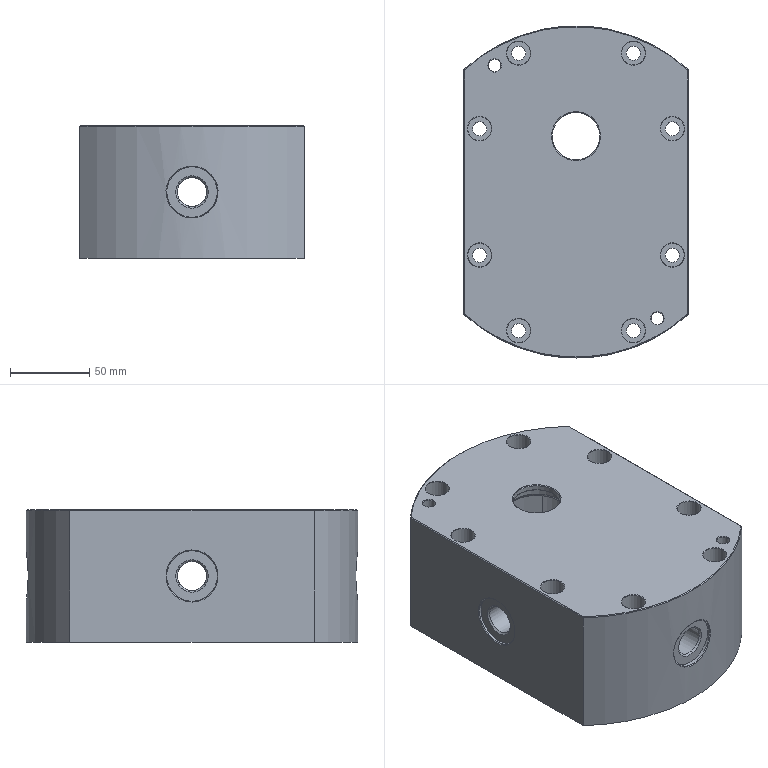NC program | NX | posted with a generic post | part box 142 x 210 x 84 mm
Lines 1 to 961 of 7150:
N10 G17 G21 G94 G90
(FLOOR_WALL_COPY_1 , TOOL : D50)
N12 T02 M6
N14 G54
N16 G17 G0 G90 X-143. Y80.997 B0. C0. S1200 M3
N18 G43 Z30. H2
N20 Z12.658
N22 G94 G1 Z9.658 F1000.
N24 X-140.
N26 X140. F2000.
N28 Y45.498
N30 X-140.
N32 Y9.999
N34 X140.
N36 Y-25.501
N38 X-140.
N40 Y-61.
N42 X140.
N44 X143.
N46 Z12.658
N48 G0 Z30.
N50 X-143. Y80.997
N52 Z12.317
N54 G1 Z9.317 F1000.
N56 X-140.
N58 X140. F2000.
N60 Y45.498
N62 X-140.
N64 Y9.999
N66 X140.
N68 Y-25.501
N70 X-140.
N72 Y-61.
N74 X140.
N76 X143.
N78 Z12.317
N80 G0 Z30.
N82 X-143. Y80.997
N84 Z11.976
N86 G1 Z8.976 F1000.
N88 X-140.
N90 X140. F2000.
N92 Y45.498
N94 X-140.
N96 Y9.999
N98 X140.
N100 Y-25.501
N102 X-140.
N104 Y-61.
N106 X140.
N108 X143.
N110 Z11.976
N112 G0 Z30.
N114 X-143. Y80.997
N116 Z11.634
N118 G1 Z8.634 F1000.
N120 X-140.
N122 X140. F2000.
N124 Y45.498
N126 X-140.
N128 Y9.999
N130 X140.
N132 Y-25.501
N134 X-140.
N136 Y-61.
N138 X140.
N140 X143.
N142 Z11.634
N144 G0 Z30.
N146 X-143. Y80.997
N148 Z11.293
N150 G1 Z8.293 F1000.
N152 X-140.
N154 X140. F2000.
N156 Y45.498
N158 X-140.
N160 Y9.999
N162 X140.
N164 Y-25.501
N166 X-140.
N168 Y-61.
N170 X140.
N172 X143.
N174 Z11.293
N176 G0 Z30.
N178 X-143. Y80.997
N180 Z10.951
N182 G1 Z7.951 F1000.
N184 X-140.
N186 X140. F2000.
N188 Y45.498
N190 X-140.
N192 Y9.999
N194 X140.
N196 Y-25.501
N198 X-140.
N200 Y-61.
N202 X140.
N204 X143.
N206 Z10.951
N208 G0 Z30.
N210 X-143. Y80.997
N212 Z10.61
N214 G1 Z7.61 F1000.
N216 X-140.
N218 X140. F2000.
N220 Y45.498
N222 X-140.
N224 Y9.999
N226 X140.
N228 Y-25.501
N230 X-140.
N232 Y-61.
N234 X140.
N236 X143.
N238 Z10.61
N240 G0 Z30.
N242 X-143. Y80.997
N244 Z10.269
N246 G1 Z7.269 F1000.
N248 X-140.
N250 X140. F2000.
N252 Y45.498
N254 X-140.
N256 Y9.999
N258 X140.
N260 Y-25.501
N262 X-140.
N264 Y-61.
N266 X140.
N268 X143.
N270 Z10.269
N272 G0 Z30.
N274 X-143. Y80.997
N276 Z9.927
N278 G1 Z6.927 F1000.
N280 X-140.
N282 X140. F2000.
N284 Y45.498
N286 X-140.
N288 Y9.999
N290 X140.
N292 Y-25.501
N294 X-140.
N296 Y-61.
N298 X140.
N300 X143.
N302 Z9.927
N304 G0 Z30.
N306 X-143. Y80.997
N308 Z9.586
N310 G1 Z6.586 F1000.
N312 X-140.
N314 X140. F2000.
N316 Y45.498
N318 X-140.
N320 Y9.999
N322 X140.
N324 Y-25.501
N326 X-140.
N328 Y-61.
N330 X140.
N332 X143.
N334 Z9.586
N336 G0 Z30.
N338 X-143. Y80.997
N340 Z9.245
N342 G1 Z6.245 F1000.
N344 X-140.
N346 X140. F2000.
N348 Y45.498
N350 X-140.
N352 Y9.999
N354 X140.
N356 Y-25.501
N358 X-140.
N360 Y-61.
N362 X140.
N364 X143.
N366 Z9.245
N368 G0 Z30.
N370 X-143. Y80.997
N372 Z8.903
N374 G1 Z5.903 F1000.
N376 X-140.
N378 X140. F2000.
N380 Y45.498
N382 X-140.
N384 Y9.999
N386 X140.
N388 Y-25.501
N390 X-140.
N392 Y-61.
N394 X140.
N396 X143.
N398 Z8.903
N400 G0 Z30.
N402 X-143. Y80.997
N404 Z8.562
N406 G1 Z5.562 F1000.
N408 X-140.
N410 X140. F2000.
N412 Y45.498
N414 X-140.
N416 Y9.999
N418 X140.
N420 Y-25.501
N422 X-140.
N424 Y-61.
N426 X140.
N428 X143.
N430 Z8.562
N432 G0 Z30.
N434 X-143. Y80.997
N436 Z8.221
N438 G1 Z5.221 F1000.
N440 X-140.
N442 X140. F2000.
N444 Y45.498
N446 X-140.
N448 Y9.999
N450 X140.
N452 Y-25.501
N454 X-140.
N456 Y-61.
N458 X140.
N460 X143.
N462 Z8.221
N464 G0 Z30.
N466 X-143. Y80.997
N468 Z7.879
N470 G1 Z4.879 F1000.
N472 X-140.
N474 X140. F2000.
N476 Y45.498
N478 X-140.
N480 Y9.999
N482 X140.
N484 Y-25.501
N486 X-140.
N488 Y-61.
N490 X140.
N492 X143.
N494 Z7.879
N496 G0 Z30.
N498 X-143. Y80.997
N500 Z7.538
N502 G1 Z4.538 F1000.
N504 X-140.
N506 X140. F2000.
N508 Y45.498
N510 X-140.
N512 Y9.999
N514 X140.
N516 Y-25.501
N518 X-140.
N520 Y-61.
N522 X140.
N524 X143.
N526 Z7.538
N528 G0 Z30.
N530 X-143. Y80.997
N532 Z7.196
N534 G1 Z4.196 F1000.
N536 X-140.
N538 X140. F2000.
N540 Y45.498
N542 X-140.
N544 Y9.999
N546 X140.
N548 Y-25.501
N550 X-140.
N552 Y-61.
N554 X140.
N556 X143.
N558 Z7.196
N560 G0 Z30.
N562 X-143. Y80.997
N564 Z6.855
N566 G1 Z3.855 F1000.
N568 X-140.
N570 X140. F2000.
N572 Y45.498
N574 X-140.
N576 Y9.999
N578 X140.
N580 Y-25.501
N582 X-140.
N584 Y-61.
N586 X140.
N588 X143.
N590 Z6.855
N592 G0 Z30.
N594 X-143. Y80.997
N596 Z6.514
N598 G1 Z3.514 F1000.
N600 X-140.
N602 X140. F2000.
N604 Y45.498
N606 X-140.
N608 Y9.999
N610 X140.
N612 Y-25.501
N614 X-140.
N616 Y-61.
N618 X140.
N620 X143.
N622 Z6.514
N624 G0 Z30.
N626 X-143. Y80.997
N628 Z6.172
N630 G1 Z3.172 F1000.
N632 X-140.
N634 X140. F2000.
N636 Y45.498
N638 X-140.
N640 Y9.999
N642 X140.
N644 Y-25.501
N646 X-140.
N648 Y-61.
N650 X140.
N652 X143.
N654 Z6.172
N656 G0 Z30.
N658 X-143. Y80.997
N660 Z5.831
N662 G1 Z2.831 F1000.
N664 X-140.
N666 X140. F2000.
N668 Y45.498
N670 X-140.
N672 Y9.999
N674 X140.
N676 Y-25.501
N678 X-140.
N680 Y-61.
N682 X140.
N684 X143.
N686 Z5.831
N688 G0 Z30.
N690 X-143. Y80.997
N692 Z5.49
N694 G1 Z2.49 F1000.
N696 X-140.
N698 X140. F2000.
N700 Y45.498
N702 X-140.
N704 Y9.999
N706 X140.
N708 Y-25.501
N710 X-140.
N712 Y-61.
N714 X140.
N716 X143.
N718 Z5.49
N720 G0 Z30.
N722 X-143. Y80.997
N724 Z5.148
N726 G1 Z2.148 F1000.
N728 X-140.
N730 X140. F2000.
N732 Y45.498
N734 X-140.
N736 Y9.999
N738 X140.
N740 Y-25.501
N742 X-140.
N744 Y-61.
N746 X140.
N748 X143.
N750 Z5.148
N752 G0 Z30.
N754 X-143. Y80.997
N756 Z4.807
N758 G1 Z1.807 F1000.
N760 X-140.
N762 X140. F2000.
N764 Y45.498
N766 X-140.
N768 Y9.999
N770 X140.
N772 Y-25.501
N774 X-140.
N776 Y-61.
N778 X140.
N780 X143.
N782 Z4.807
N784 G0 Z30.
N786 X-143. Y80.997
N788 Z4.465
N790 G1 Z1.465 F1000.
N792 X-140.
N794 X140. F2000.
N796 Y45.498
N798 X-140.
N800 Y9.999
N802 X140.
N804 Y-25.501
N806 X-140.
N808 Y-61.
N810 X140.
N812 X143.
N814 Z4.465
N816 G0 Z30.
N818 X-143. Y80.997
N820 Z4.124
N822 G1 Z1.124 F1000.
N824 X-140.
N826 X140. F2000.
N828 Y45.498
N830 X-140.
N832 Y9.999
N834 X140.
N836 Y-25.501
N838 X-140.
N840 Y-61.
N842 X140.
N844 X143.
N846 Z4.124
N848 G0 Z30.
N850 X-143. Y80.997
N852 Z3.783
N854 G1 Z0.783 F1000.
N856 X-140.
N858 X140. F2000.
N860 Y45.498
N862 X-140.
N864 Y9.999
N866 X140.
N868 Y-25.501
N870 X-140.
N872 Y-61.
N874 X140.
N876 X143.
N878 Z3.783
N880 G0 Z30.
N882 X-143. Y80.997
N884 Z3.441
N886 G1 Z0.441 F1000.
N888 X-140.
N890 X140. F2000.
N892 Y45.498
N894 X-140.
N896 Y9.999
N898 X140.
N900 Y-25.501
N902 X-140.
N904 Y-61.
N906 X140.
N908 X143.
N910 Z3.441
N912 G0 Z30.
N914 X-143. Y80.997
N916 Z3.1
N918 G1 Z0.1 F1000.
N920 X-140.
N922 X140. F2000.
N924 Y45.498
N926 X-140.
N928 Y9.999
N930 X140.
N932 Y-25.501
N934 X-140.
N936 Y-61.
N938 X140.
N940 X143.
N942 Z3.1
N944 G0 Z30.
(FLOOR_WALL_COPY_COPY , TOOL : D50)
N946 X-143. Y80.997 S2500
N948 Z3.
N950 G1 Z0. F1000.
N952 X-140.
N954 X140.
N956 Y45.498
N958 X-140.
N960 Y9.999
N962 X140.
N964 Y-25.501
N966 X-140.
N968 Y-61.
N970 X140.
N972 X143.
N974 Z3.
N976 G0 Z30.
N978 M5
(DRILLING_COPY_1 , TOOL : ZXZ)
N980 T01 M6
N982 G54
N984 G17 G0 G90 X-40. Y-61. B0. C0. S5000 M3
N986 G43 Z30. H1
N988 G94 G81 G98 Z-1. F250. R3.
N990 X-87.769 Y-36.355
N992 Y36.355
N994 X-80. Y51.5
N996 X-40. Y61.
N998 X40.
N1000 X87.769 Y36.355
N1002 Y-36.355
N1004 X80. Y-51.5
N1006 X40. Y-61.
N1008 G80
N1010 G0 X40. Y-61. Z30.
N1012 M5
(DRILLING_COPY , TOOL : 9.0ZT)
N1014 T09 M6
N1016 G54
N1018 G17 G0 G90 X40. Y-61. B0. C0. S2000 M3
N1020 G43 Z30. H9
N1022 G94 G83 G98 Z-53.204 F150. Q2. R3.
N1024 X87.769 Y-36.355
N1026 Y36.355
N1028 X40. Y61.
N1030 X-40.
N1032 X-87.769 Y36.355
N1034 Y-36.355
N1036 X-40. Y-61.
N1038 G80
N1040 G0 X-40. Y-61. Z30.
N1042 M5
(DRILLING_COPY_COPY , TOOL : 7.8ZT)
N1044 T08 M6
N1046 G54
N1048 G17 G0 G90 X-80. Y51.5 B0. C0. S2000 M3
N1050 G43 Z30. H8
N1052 G94 G83 G98 Z-23.343 F150. Q2. R3.
N1054 X80. Y-51.5
N1056 G80
N1058 G0 X80. Y-51.5 Z30.
N1060 M5
(DRILLING_COPY_COPY_COPY , TOOL : 8.0JD)
N1062 T18 M6
N1064 G54
N1066 G17 G0 G90 X-80. Y51.5 B0. C0. S800 M3
N1068 G43 Z30. H18
N1070 G94 G85 G98 Z-20. F40. R3.
N1072 X80. Y-51.5
N1074 G80
N1076 G0 X80. Y-51.5 Z30.
N1078 M5
(PLANAR_PROFILE , TOOL : D3)
N1080 T03 M6
N1082 G54
N1084 G17 G0 G90 X0. Y53.5 B0. C0. S5000 M3
N1086 G43 Z30. H3
N1088 Z3.
N1090 G94 G1 Z-0.05 F500.
N1092 X58.89 F1100.
N1094 G2 X75.777 Y43.75 R19.5
N1096 X75.777 Y-43.75 R87.5
N1098 X58.89 Y-53.5 R19.5
N1100 G1 X-58.89
N1102 G2 X-75.777 Y-43.75 R19.5
N1104 X-75.777 Y43.75 R87.5
N1106 X-58.89 Y53.5 R19.5
N1108 G1 X0.
N1110 Z2.95
N1112 Z-0.1 F500.
N1114 X-58.89 F1100.
N1116 G3 X-75.777 Y43.75 R19.5
N1118 X-75.777 Y-43.75 R87.5
N1120 X-58.89 Y-53.5 R19.5
N1122 G1 X58.89
N1124 G3 X75.777 Y-43.75 R19.5
N1126 X75.777 Y43.75 R87.5
N1128 X58.89 Y53.5 R19.5
N1130 G1 X0.
N1132 Z2.9
N1134 Z-0.15 F500.
N1136 X58.89 F1100.
N1138 G2 X75.777 Y43.75 R19.5
N1140 X75.777 Y-43.75 R87.5
N1142 X58.89 Y-53.5 R19.5
N1144 G1 X-58.89
N1146 G2 X-75.777 Y-43.75 R19.5
N1148 X-75.777 Y43.75 R87.5
N1150 X-58.89 Y53.5 R19.5
N1152 G1 X0.
N1154 Z2.85
N1156 Z-0.2 F500.
N1158 X-58.89 F1100.
N1160 G3 X-75.777 Y43.75 R19.5
N1162 X-75.777 Y-43.75 R87.5
N1164 X-58.89 Y-53.5 R19.5
N1166 G1 X58.89
N1168 G3 X75.777 Y-43.75 R19.5
N1170 X75.777 Y43.75 R87.5
N1172 X58.89 Y53.5 R19.5
N1174 G1 X0.
N1176 Z2.8
N1178 Z-0.25 F500.
N1180 X58.89 F1100.
N1182 G2 X75.777 Y43.75 R19.5
N1184 X75.777 Y-43.75 R87.5
N1186 X58.89 Y-53.5 R19.5
N1188 G1 X-58.89
N1190 G2 X-75.777 Y-43.75 R19.5
N1192 X-75.777 Y43.75 R87.5
N1194 X-58.89 Y53.5 R19.5
N1196 G1 X0.
N1198 Z2.75
N1200 Z-0.3 F500.
N1202 X-58.89 F1100.
N1204 G3 X-75.777 Y43.75 R19.5
N1206 X-75.777 Y-43.75 R87.5
N1208 X-58.89 Y-53.5 R19.5
N1210 G1 X58.89
N1212 G3 X75.777 Y-43.75 R19.5
N1214 X75.777 Y43.75 R87.5
N1216 X58.89 Y53.5 R19.5
N1218 G1 X0.
N1220 Z2.7
N1222 Z-0.35 F500.
N1224 X58.89 F1100.
N1226 G2 X75.777 Y43.75 R19.5
N1228 X75.777 Y-43.75 R87.5
N1230 X58.89 Y-53.5 R19.5
N1232 G1 X-58.89
N1234 G2 X-75.777 Y-43.75 R19.5
N1236 X-75.777 Y43.75 R87.5
N1238 X-58.89 Y53.5 R19.5
N1240 G1 X0.
N1242 Z2.65
N1244 Z-0.4 F500.
N1246 X-58.89 F1100.
N1248 G3 X-75.777 Y43.75 R19.5
N1250 X-75.777 Y-43.75 R87.5
N1252 X-58.89 Y-53.5 R19.5
N1254 G1 X58.89
N1256 G3 X75.777 Y-43.75 R19.5
N1258 X75.777 Y43.75 R87.5
N1260 X58.89 Y53.5 R19.5
N1262 G1 X0.
N1264 Z2.6
N1266 Z-0.45 F500.
N1268 X58.89 F1100.
N1270 G2 X75.777 Y43.75 R19.5
N1272 X75.777 Y-43.75 R87.5
N1274 X58.89 Y-53.5 R19.5
N1276 G1 X-58.89
N1278 G2 X-75.777 Y-43.75 R19.5
N1280 X-75.777 Y43.75 R87.5
N1282 X-58.89 Y53.5 R19.5
N1284 G1 X0.
N1286 Z2.55
N1288 Z-0.5 F500.
N1290 X-58.89 F1100.
N1292 G3 X-75.777 Y43.75 R19.5
N1294 X-75.777 Y-43.75 R87.5
N1296 X-58.89 Y-53.5 R19.5
N1298 G1 X58.89
N1300 G3 X75.777 Y-43.75 R19.5
N1302 X75.777 Y43.75 R87.5
N1304 X58.89 Y53.5 R19.5
N1306 G1 X0.
N1308 Z2.5
N1310 Z-0.55 F500.
N1312 X58.89 F1100.
N1314 G2 X75.777 Y43.75 R19.5
N1316 X75.777 Y-43.75 R87.5
N1318 X58.89 Y-53.5 R19.5
N1320 G1 X-58.89
N1322 G2 X-75.777 Y-43.75 R19.5
N1324 X-75.777 Y43.75 R87.5
N1326 X-58.89 Y53.5 R19.5
N1328 G1 X0.
N1330 Z2.45
N1332 Z-0.6 F500.
N1334 X-58.89 F1100.
N1336 G3 X-75.777 Y43.75 R19.5
N1338 X-75.777 Y-43.75 R87.5
N1340 X-58.89 Y-53.5 R19.5
N1342 G1 X58.89
N1344 G3 X75.777 Y-43.75 R19.5
N1346 X75.777 Y43.75 R87.5
N1348 X58.89 Y53.5 R19.5
N1350 G1 X0.
N1352 Z2.4
N1354 Z-0.65 F500.
N1356 X58.89 F1100.
N1358 G2 X75.777 Y43.75 R19.5
N1360 X75.777 Y-43.75 R87.5
N1362 X58.89 Y-53.5 R19.5
N1364 G1 X-58.89
N1366 G2 X-75.777 Y-43.75 R19.5
N1368 X-75.777 Y43.75 R87.5
N1370 X-58.89 Y53.5 R19.5
N1372 G1 X0.
N1374 Z2.35
N1376 Z-0.7 F500.
N1378 X-58.89 F1100.
N1380 G3 X-75.777 Y43.75 R19.5
N1382 X-75.777 Y-43.75 R87.5
N1384 X-58.89 Y-53.5 R19.5
N1386 G1 X58.89
N1388 G3 X75.777 Y-43.75 R19.5
N1390 X75.777 Y43.75 R87.5
N1392 X58.89 Y53.5 R19.5
N1394 G1 X0.
N1396 Z2.3
N1398 Z-0.75 F500.
N1400 X58.89 F1100.
N1402 G2 X75.777 Y43.75 R19.5
N1404 X75.777 Y-43.75 R87.5
N1406 X58.89 Y-53.5 R19.5
N1408 G1 X-58.89
N1410 G2 X-75.777 Y-43.75 R19.5
N1412 X-75.777 Y43.75 R87.5
N1414 X-58.89 Y53.5 R19.5
N1416 G1 X0.
N1418 Z2.25
N1420 Z-0.8 F500.
N1422 X-58.89 F1100.
N1424 G3 X-75.777 Y43.75 R19.5
N1426 X-75.777 Y-43.75 R87.5
N1428 X-58.89 Y-53.5 R19.5
N1430 G1 X58.89
N1432 G3 X75.777 Y-43.75 R19.5
N1434 X75.777 Y43.75 R87.5
N1436 X58.89 Y53.5 R19.5
N1438 G1 X0.
N1440 Z2.2
N1442 Z-0.85 F500.
N1444 X58.89 F1100.
N1446 G2 X75.777 Y43.75 R19.5
N1448 X75.777 Y-43.75 R87.5
N1450 X58.89 Y-53.5 R19.5
N1452 G1 X-58.89
N1454 G2 X-75.777 Y-43.75 R19.5
N1456 X-75.777 Y43.75 R87.5
N1458 X-58.89 Y53.5 R19.5
N1460 G1 X0.
N1462 Z2.15
N1464 Z-0.9 F500.
N1466 X-58.89 F1100.
N1468 G3 X-75.777 Y43.75 R19.5
N1470 X-75.777 Y-43.75 R87.5
N1472 X-58.89 Y-53.5 R19.5
N1474 G1 X58.89
N1476 G3 X75.777 Y-43.75 R19.5
N1478 X75.777 Y43.75 R87.5
N1480 X58.89 Y53.5 R19.5
N1482 G1 X0.
N1484 Z2.1
N1486 Z-0.95 F500.
N1488 X58.89 F1100.
N1490 G2 X75.777 Y43.75 R19.5
N1492 X75.777 Y-43.75 R87.5
N1494 X58.89 Y-53.5 R19.5
N1496 G1 X-58.89
N1498 G2 X-75.777 Y-43.75 R19.5
N1500 X-75.777 Y43.75 R87.5
N1502 X-58.89 Y53.5 R19.5
N1504 G1 X0.
N1506 Z2.05
N1508 Z-1. F500.
N1510 X-58.89 F1100.
N1512 G3 X-75.777 Y43.75 R19.5
N1514 X-75.777 Y-43.75 R87.5
N1516 X-58.89 Y-53.5 R19.5
N1518 G1 X58.89
N1520 G3 X75.777 Y-43.75 R19.5
N1522 X75.777 Y43.75 R87.5
N1524 X58.89 Y53.5 R19.5
N1526 G1 X0.
N1528 Z2.
N1530 Z-1.05 F500.
N1532 X58.89 F1100.
N1534 G2 X75.777 Y43.75 R19.5
N1536 X75.777 Y-43.75 R87.5
N1538 X58.89 Y-53.5 R19.5
N1540 G1 X-58.89
N1542 G2 X-75.777 Y-43.75 R19.5
N1544 X-75.777 Y43.75 R87.5
N1546 X-58.89 Y53.5 R19.5
N1548 G1 X0.
N1550 Z1.95
N1552 Z-1.1 F500.
N1554 X-58.89 F1100.
N1556 G3 X-75.777 Y43.75 R19.5
N1558 X-75.777 Y-43.75 R87.5
N1560 X-58.89 Y-53.5 R19.5
N1562 G1 X58.89
N1564 G3 X75.777 Y-43.75 R19.5
N1566 X75.777 Y43.75 R87.5
N1568 X58.89 Y53.5 R19.5
N1570 G1 X0.
N1572 Z1.9
N1574 Z-1.15 F500.
N1576 X58.89 F1100.
N1578 G2 X75.777 Y43.75 R19.5
N1580 X75.777 Y-43.75 R87.5
N1582 X58.89 Y-53.5 R19.5
N1584 G1 X-58.89
N1586 G2 X-75.777 Y-43.75 R19.5
N1588 X-75.777 Y43.75 R87.5
N1590 X-58.89 Y53.5 R19.5
N1592 G1 X0.
N1594 Z1.85
N1596 Z-1.2 F500.
N1598 X-58.89 F1100.
N1600 G3 X-75.777 Y43.75 R19.5
N1602 X-75.777 Y-43.75 R87.5
N1604 X-58.89 Y-53.5 R19.5
N1606 G1 X58.89
N1608 G3 X75.777 Y-43.75 R19.5
N1610 X75.777 Y43.75 R87.5
N1612 X58.89 Y53.5 R19.5
N1614 G1 X0.
N1616 Z1.8
N1618 Z-1.25 F500.
N1620 X58.89 F1100.
N1622 G2 X75.777 Y43.75 R19.5
N1624 X75.777 Y-43.75 R87.5
N1626 X58.89 Y-53.5 R19.5
N1628 G1 X-58.89
N1630 G2 X-75.777 Y-43.75 R19.5
N1632 X-75.777 Y43.75 R87.5
N1634 X-58.89 Y53.5 R19.5
N1636 G1 X0.
N1638 Z1.75
N1640 Z-1.3 F500.
N1642 X-58.89 F1100.
N1644 G3 X-75.777 Y43.75 R19.5
N1646 X-75.777 Y-43.75 R87.5
N1648 X-58.89 Y-53.5 R19.5
N1650 G1 X58.89
N1652 G3 X75.777 Y-43.75 R19.5
N1654 X75.777 Y43.75 R87.5
N1656 X58.89 Y53.5 R19.5
N1658 G1 X0.
N1660 Z1.7
N1662 Z-1.35 F500.
N1664 X58.89 F1100.
N1666 G2 X75.777 Y43.75 R19.5
N1668 X75.777 Y-43.75 R87.5
N1670 X58.89 Y-53.5 R19.5
N1672 G1 X-58.89
N1674 G2 X-75.777 Y-43.75 R19.5
N1676 X-75.777 Y43.75 R87.5
N1678 X-58.89 Y53.5 R19.5
N1680 G1 X0.
N1682 Z1.65
N1684 Z-1.4 F500.
N1686 X-58.89 F1100.
N1688 G3 X-75.777 Y43.75 R19.5
N1690 X-75.777 Y-43.75 R87.5
N1692 X-58.89 Y-53.5 R19.5
N1694 G1 X58.89
N1696 G3 X75.777 Y-43.75 R19.5
N1698 X75.777 Y43.75 R87.5
N1700 X58.89 Y53.5 R19.5
N1702 G1 X0.
N1704 Z1.6
N1706 Z-1.45 F500.
N1708 X58.89 F1100.
N1710 G2 X75.777 Y43.75 R19.5
N1712 X75.777 Y-43.75 R87.5
N1714 X58.89 Y-53.5 R19.5
N1716 G1 X-58.89
N1718 G2 X-75.777 Y-43.75 R19.5
N1720 X-75.777 Y43.75 R87.5
N1722 X-58.89 Y53.5 R19.5
N1724 G1 X0.
N1726 Z1.55
N1728 Z-1.5 F500.
N1730 X-58.89 F1100.
N1732 G3 X-75.777 Y43.75 R19.5
N1734 X-75.777 Y-43.75 R87.5
N1736 X-58.89 Y-53.5 R19.5
N1738 G1 X58.89
N1740 G3 X75.777 Y-43.75 R19.5
N1742 X75.777 Y43.75 R87.5
N1744 X58.89 Y53.5 R19.5
N1746 G1 X0.
N1748 Z1.5
N1750 Z-1.55 F500.
N1752 X58.89 F1100.
N1754 G2 X75.777 Y43.75 R19.5
N1756 X75.777 Y-43.75 R87.5
N1758 X58.89 Y-53.5 R19.5
N1760 G1 X-58.89
N1762 G2 X-75.777 Y-43.75 R19.5
N1764 X-75.777 Y43.75 R87.5
N1766 X-58.89 Y53.5 R19.5
N1768 G1 X0.
N1770 Z1.45
N1772 Z-1.6 F500.
N1774 X-58.89 F1100.
N1776 G3 X-75.777 Y43.75 R19.5
N1778 X-75.777 Y-43.75 R87.5
N1780 X-58.89 Y-53.5 R19.5
N1782 G1 X58.89
N1784 G3 X75.777 Y-43.75 R19.5
N1786 X75.777 Y43.75 R87.5
N1788 X58.89 Y53.5 R19.5
N1790 G1 X0.
N1792 Z1.4
N1794 Z-1.65 F500.
N1796 X58.89 F1100.
N1798 G2 X75.777 Y43.75 R19.5
N1800 X75.777 Y-43.75 R87.5
N1802 X58.89 Y-53.5 R19.5
N1804 G1 X-58.89
N1806 G2 X-75.777 Y-43.75 R19.5
N1808 X-75.777 Y43.75 R87.5
N1810 X-58.89 Y53.5 R19.5
N1812 G1 X0.
N1814 Z1.35
N1816 Z-1.7 F500.
N1818 X-58.89 F1100.
N1820 G3 X-75.777 Y43.75 R19.5
N1822 X-75.777 Y-43.75 R87.5
N1824 X-58.89 Y-53.5 R19.5
N1826 G1 X58.89
N1828 G3 X75.777 Y-43.75 R19.5
N1830 X75.777 Y43.75 R87.5
N1832 X58.89 Y53.5 R19.5
N1834 G1 X0.
N1836 Z1.3
N1838 Z-1.75 F500.
N1840 X58.89 F1100.
N1842 G2 X75.777 Y43.75 R19.5
N1844 X75.777 Y-43.75 R87.5
N1846 X58.89 Y-53.5 R19.5
N1848 G1 X-58.89
N1850 G2 X-75.777 Y-43.75 R19.5
N1852 X-75.777 Y43.75 R87.5
N1854 X-58.89 Y53.5 R19.5
N1856 G1 X0.
N1858 Z1.25
N1860 Z-1.8 F500.
N1862 X-58.89 F1100.
N1864 G3 X-75.777 Y43.75 R19.5
N1866 X-75.777 Y-43.75 R87.5
N1868 X-58.89 Y-53.5 R19.5
N1870 G1 X58.89
N1872 G3 X75.777 Y-43.75 R19.5
N1874 X75.777 Y43.75 R87.5
N1876 X58.89 Y53.5 R19.5
N1878 G1 X0.
N1880 Z1.2
N1882 G0 Z30.
N1884 M5